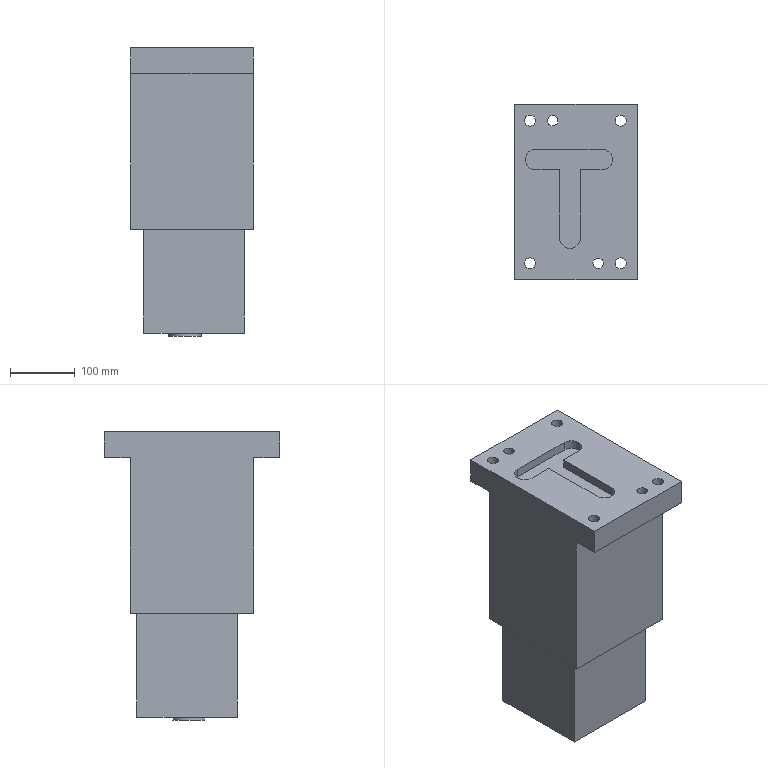Part | NX | features solid 2 | 1 solid | 42 faces | box 188.25 x 270 x 445 mm | volume 14281883 mm3 | plane 26 | cylinder 15 | cone 1 | commonest cylinder face diameters 17 x4 25 x4 32 x3 16 x2 20 x1 50 x1
STEP:
#1=CARTESIAN_POINT('',(-1140.,-620.,130.));
#2=VERTEX_POINT('',#1);
#3=CARTESIAN_POINT('',(-1140.,-350.,130.));
#4=VERTEX_POINT('',#3);
#5=CARTESIAN_POINT('',(-1140.,-555.,130.));
#6=DIRECTION('',(0.,-1.,0.));
#7=VECTOR('',#6,1000.);
#8=LINE('',#5,#7);
#9=EDGE_CURVE('',#2,#4,#8,.F.);
#10=ORIENTED_EDGE('',*,*,#9,.F.);
#11=CARTESIAN_POINT('',(-951.75,-620.,130.));
#12=VERTEX_POINT('',#11);
#13=CARTESIAN_POINT('',(-1136.75,-620.,130.));
#14=DIRECTION('',(1.,0.,0.));
#15=VECTOR('',#14,1000.);
#16=LINE('',#13,#15);
#17=EDGE_CURVE('',#2,#12,#16,.T.);
#18=ORIENTED_EDGE('',*,*,#17,.T.);
#19=CARTESIAN_POINT('',(-951.75,-350.,130.));
#20=VERTEX_POINT('',#19);
#21=CARTESIAN_POINT('',(-951.75,-564.335,130.));
#22=DIRECTION('',(0.,1.,0.));
#23=VECTOR('',#22,1000.);
#24=LINE('',#21,#23);
#25=EDGE_CURVE('',#12,#20,#24,.T.);
#26=ORIENTED_EDGE('',*,*,#25,.T.);
#27=CARTESIAN_POINT('',(-1136.75,-350.,130.));
#28=DIRECTION('',(-1.,0.,0.));
#29=VECTOR('',#28,1000.);
#30=LINE('',#27,#29);
#31=EDGE_CURVE('',#20,#4,#30,.T.);
#32=ORIENTED_EDGE('',*,*,#31,.T.);
#33=EDGE_LOOP('',(#10,#18,#26,#32));
#34=FACE_BOUND('',#33,.T.);
#35=CARTESIAN_POINT('',(-1019.75,-595.,130.));
#36=VERTEX_POINT('',#35);
#37=CARTESIAN_POINT('',(-1011.75,-595.,130.));
#38=DIRECTION('',(0.,0.,-1.));
#39=DIRECTION('',(-1.,0.,0.));
#40=AXIS2_PLACEMENT_3D('',#37,#38,#39);
#41=CIRCLE('',#40,8.);
#42=EDGE_CURVE('',#36,#36,#41,.T.);
#43=ORIENTED_EDGE('',*,*,#42,.T.);
#44=EDGE_LOOP('',(#43));
#45=FACE_BOUND('',#44,.T.);
#46=CARTESIAN_POINT('',(-985.25,-595.,130.));
#47=VERTEX_POINT('',#46);
#48=CARTESIAN_POINT('',(-976.75,-595.,130.));
#49=DIRECTION('',(0.,0.,-1.));
#50=DIRECTION('',(-1.,0.,0.));
#51=AXIS2_PLACEMENT_3D('',#48,#49,#50);
#52=CIRCLE('',#51,8.5);
#53=EDGE_CURVE('',#47,#47,#52,.T.);
#54=ORIENTED_EDGE('',*,*,#53,.T.);
#55=EDGE_LOOP('',(#54));
#56=FACE_BOUND('',#55,.T.);
#57=CARTESIAN_POINT('',(-985.25,-375.,130.));
#58=VERTEX_POINT('',#57);
#59=CARTESIAN_POINT('',(-976.75,-375.,130.));
#60=DIRECTION('',(0.,0.,-1.));
#61=DIRECTION('',(-1.,0.,0.));
#62=AXIS2_PLACEMENT_3D('',#59,#60,#61);
#63=CIRCLE('',#62,8.5);
#64=EDGE_CURVE('',#58,#58,#63,.T.);
#65=ORIENTED_EDGE('',*,*,#64,.T.);
#66=EDGE_LOOP('',(#65));
#67=FACE_BOUND('',#66,.T.);
#68=CARTESIAN_POINT('',(-1071.,-556.,130.));
#69=VERTEX_POINT('',#68);
#70=CARTESIAN_POINT('',(-1071.,-451.,130.));
#71=VERTEX_POINT('',#70);
#72=CARTESIAN_POINT('',(-1071.,-564.335,130.));
#73=DIRECTION('',(0.,-1.,0.));
#74=VECTOR('',#73,1000.);
#75=LINE('',#72,#74);
#76=EDGE_CURVE('',#69,#71,#75,.F.);
#77=ORIENTED_EDGE('',*,*,#76,.T.);
#78=CARTESIAN_POINT('',(-1107.75,-451.,130.));
#79=VERTEX_POINT('',#78);
#80=CARTESIAN_POINT('',(-1061.75,-451.,130.));
#81=DIRECTION('',(1.,0.,0.));
#82=VECTOR('',#81,1000.);
#83=LINE('',#80,#82);
#84=EDGE_CURVE('',#79,#71,#83,.T.);
#85=ORIENTED_EDGE('',*,*,#84,.F.);
#86=CARTESIAN_POINT('',(-1107.75,-419.,130.));
#87=VERTEX_POINT('',#86);
#88=CARTESIAN_POINT('',(-1107.75,-435.,130.));
#89=DIRECTION('',(0.,0.,-1.));
#90=DIRECTION('',(-1.,0.,0.));
#91=AXIS2_PLACEMENT_3D('',#88,#89,#90);
#92=CIRCLE('',#91,16.);
#93=EDGE_CURVE('',#79,#87,#92,.T.);
#94=ORIENTED_EDGE('',*,*,#93,.T.);
#95=CARTESIAN_POINT('',(-1005.75,-419.,130.));
#96=VERTEX_POINT('',#95);
#97=CARTESIAN_POINT('',(-1126.75,-419.,130.));
#98=DIRECTION('',(1.,0.,0.));
#99=VECTOR('',#98,1000.);
#100=LINE('',#97,#99);
#101=EDGE_CURVE('',#87,#96,#100,.T.);
#102=ORIENTED_EDGE('',*,*,#101,.T.);
#103=CARTESIAN_POINT('',(-1005.75,-451.,130.));
#104=VERTEX_POINT('',#103);
#105=CARTESIAN_POINT('',(-1005.75,-435.,130.));
#106=DIRECTION('',(0.,0.,-1.));
#107=DIRECTION('',(-1.,0.,0.));
#108=AXIS2_PLACEMENT_3D('',#105,#106,#107);
#109=CIRCLE('',#108,16.);
#110=EDGE_CURVE('',#96,#104,#109,.T.);
#111=ORIENTED_EDGE('',*,*,#110,.T.);
#112=CARTESIAN_POINT('',(-1039.,-451.,130.));
#113=VERTEX_POINT('',#112);
#114=CARTESIAN_POINT('',(-1061.75,-451.,130.));
#115=DIRECTION('',(1.,0.,0.));
#116=VECTOR('',#115,1000.);
#117=LINE('',#114,#116);
#118=EDGE_CURVE('',#113,#104,#117,.T.);
#119=ORIENTED_EDGE('',*,*,#118,.F.);
#120=CARTESIAN_POINT('',(-1039.,-556.,130.));
#121=VERTEX_POINT('',#120);
#122=CARTESIAN_POINT('',(-1039.,-564.335,130.));
#123=DIRECTION('',(0.,-1.,0.));
#124=VECTOR('',#123,1000.);
#125=LINE('',#122,#124);
#126=EDGE_CURVE('',#113,#121,#125,.T.);
#127=ORIENTED_EDGE('',*,*,#126,.T.);
#128=CARTESIAN_POINT('',(-1055.,-556.,130.));
#129=DIRECTION('',(0.,0.,-1.));
#130=DIRECTION('',(-1.,0.,0.));
#131=AXIS2_PLACEMENT_3D('',#128,#129,#130);
#132=CIRCLE('',#131,16.);
#133=EDGE_CURVE('',#69,#121,#132,.F.);
#134=ORIENTED_EDGE('',*,*,#133,.F.);
#135=EDGE_LOOP('',(#77,#85,#94,#102,#111,#119,#127,#134));
#136=FACE_BOUND('',#135,.T.);
#137=CARTESIAN_POINT('',(-1125.25,-595.,130.));
#138=VERTEX_POINT('',#137);
#139=CARTESIAN_POINT('',(-1116.75,-595.,130.));
#140=DIRECTION('',(0.,0.,-1.));
#141=DIRECTION('',(-1.,0.,0.));
#142=AXIS2_PLACEMENT_3D('',#139,#140,#141);
#143=CIRCLE('',#142,8.5);
#144=EDGE_CURVE('',#138,#138,#143,.T.);
#145=ORIENTED_EDGE('',*,*,#144,.T.);
#146=EDGE_LOOP('',(#145));
#147=FACE_BOUND('',#146,.T.);
#148=CARTESIAN_POINT('',(-1125.25,-375.,130.));
#149=VERTEX_POINT('',#148);
#150=CARTESIAN_POINT('',(-1116.75,-375.,130.));
#151=DIRECTION('',(0.,0.,-1.));
#152=DIRECTION('',(-1.,0.,0.));
#153=AXIS2_PLACEMENT_3D('',#150,#151,#152);
#154=CIRCLE('',#153,8.5);
#155=EDGE_CURVE('',#149,#149,#154,.T.);
#156=ORIENTED_EDGE('',*,*,#155,.T.);
#157=EDGE_LOOP('',(#156));
#158=FACE_BOUND('',#157,.T.);
#159=CARTESIAN_POINT('',(-1073.75,-375.,130.));
#160=VERTEX_POINT('',#159);
#161=CARTESIAN_POINT('',(-1081.75,-375.,130.));
#162=DIRECTION('',(0.,0.,1.));
#163=DIRECTION('',(1.,0.,0.));
#164=AXIS2_PLACEMENT_3D('',#161,#162,#163);
#165=CIRCLE('',#164,8.);
#166=EDGE_CURVE('',#160,#160,#165,.F.);
#167=ORIENTED_EDGE('',*,*,#166,.T.);
#168=EDGE_LOOP('',(#167));
#169=FACE_BOUND('',#168,.T.);
#170=CARTESIAN_POINT('',(-1136.75,-564.335,130.));
#171=DIRECTION('',(0.,0.,1.));
#172=DIRECTION('',(0.,-1.,0.));
#173=AXIS2_PLACEMENT_3D('',#170,#171,#172);
#174=PLANE('',#173);
#175=ADVANCED_FACE('',(#34,#45,#56,#67,#136,#147,#158,#169),#174,.T.);
#176=CARTESIAN_POINT('',(-951.75,-350.,90.));
#177=VERTEX_POINT('',#176);
#178=CARTESIAN_POINT('',(-951.75,-390.,90.));
#179=VERTEX_POINT('',#178);
#180=CARTESIAN_POINT('',(-951.75,-484.335,90.));
#181=DIRECTION('',(0.,-1.,0.));
#182=VECTOR('',#181,1000.);
#183=LINE('',#180,#182);
#184=EDGE_CURVE('',#177,#179,#183,.T.);
#185=ORIENTED_EDGE('',*,*,#184,.T.);
#186=CARTESIAN_POINT('',(-1140.,-390.,90.));
#187=VERTEX_POINT('',#186);
#188=CARTESIAN_POINT('',(-974.25,-390.,90.));
#189=DIRECTION('',(-1.,0.,0.));
#190=VECTOR('',#189,1000.);
#191=LINE('',#188,#190);
#192=EDGE_CURVE('',#179,#187,#191,.T.);
#193=ORIENTED_EDGE('',*,*,#192,.T.);
#194=CARTESIAN_POINT('',(-1140.,-350.,90.));
#195=VERTEX_POINT('',#194);
#196=CARTESIAN_POINT('',(-1140.,-555.,90.));
#197=DIRECTION('',(0.,1.,0.));
#198=VECTOR('',#197,1000.);
#199=LINE('',#196,#198);
#200=EDGE_CURVE('',#195,#187,#199,.F.);
#201=ORIENTED_EDGE('',*,*,#200,.F.);
#202=CARTESIAN_POINT('',(-974.25,-350.,90.));
#203=DIRECTION('',(-1.,0.,0.));
#204=VECTOR('',#203,1000.);
#205=LINE('',#202,#204);
#206=EDGE_CURVE('',#177,#195,#205,.T.);
#207=ORIENTED_EDGE('',*,*,#206,.F.);
#208=EDGE_LOOP('',(#185,#193,#201,#207));
#209=FACE_BOUND('',#208,.T.);
#210=CARTESIAN_POINT('',(-989.25,-375.,90.));
#211=VERTEX_POINT('',#210);
#212=CARTESIAN_POINT('',(-976.75,-375.,90.));
#213=DIRECTION('',(0.,0.,-1.));
#214=DIRECTION('',(-1.,0.,0.));
#215=AXIS2_PLACEMENT_3D('',#212,#213,#214);
#216=CIRCLE('',#215,12.5);
#217=EDGE_CURVE('',#211,#211,#216,.T.);
#218=ORIENTED_EDGE('',*,*,#217,.F.);
#219=EDGE_LOOP('',(#218));
#220=FACE_BOUND('',#219,.T.);
#221=CARTESIAN_POINT('',(-1104.25,-375.,90.));
#222=VERTEX_POINT('',#221);
#223=CARTESIAN_POINT('',(-1116.75,-375.,90.));
#224=DIRECTION('',(0.,0.,1.));
#225=DIRECTION('',(1.,0.,0.));
#226=AXIS2_PLACEMENT_3D('',#223,#224,#225);
#227=CIRCLE('',#226,12.5);
#228=EDGE_CURVE('',#222,#222,#227,.T.);
#229=ORIENTED_EDGE('',*,*,#228,.T.);
#230=EDGE_LOOP('',(#229));
#231=FACE_BOUND('',#230,.T.);
#232=CARTESIAN_POINT('',(-1089.75,-375.,90.));
#233=VERTEX_POINT('',#232);
#234=CARTESIAN_POINT('',(-1081.75,-375.,90.));
#235=DIRECTION('',(0.,0.,-1.));
#236=DIRECTION('',(-1.,0.,0.));
#237=AXIS2_PLACEMENT_3D('',#234,#235,#236);
#238=CIRCLE('',#237,8.);
#239=EDGE_CURVE('',#233,#233,#238,.F.);
#240=ORIENTED_EDGE('',*,*,#239,.T.);
#241=EDGE_LOOP('',(#240));
#242=FACE_BOUND('',#241,.T.);
#243=CARTESIAN_POINT('',(-974.25,-484.335,90.));
#244=DIRECTION('',(0.,0.,-1.));
#245=DIRECTION('',(-1.,0.,0.));
#246=AXIS2_PLACEMENT_3D('',#243,#244,#245);
#247=PLANE('',#246);
#248=ADVANCED_FACE('',(#209,#220,#231,#242),#247,.T.);
#249=CARTESIAN_POINT('',(-1120.,-400.,-150.));
#250=VERTEX_POINT('',#249);
#251=CARTESIAN_POINT('',(-965.,-400.,-150.));
#252=VERTEX_POINT('',#251);
#253=CARTESIAN_POINT('',(-861.25,-400.,-150.));
#254=DIRECTION('',(-1.,0.,0.));
#255=VECTOR('',#254,1000.);
#256=LINE('',#253,#255);
#257=EDGE_CURVE('',#250,#252,#256,.F.);
#258=ORIENTED_EDGE('',*,*,#257,.T.);
#259=CARTESIAN_POINT('',(-965.,-400.,-310.));
#260=VERTEX_POINT('',#259);
#261=CARTESIAN_POINT('',(-965.,-400.,-100.));
#262=DIRECTION('',(0.,0.,-1.));
#263=VECTOR('',#262,1000.);
#264=LINE('',#261,#263);
#265=EDGE_CURVE('',#252,#260,#264,.T.);
#266=ORIENTED_EDGE('',*,*,#265,.T.);
#267=CARTESIAN_POINT('',(-1120.,-400.,-310.));
#268=VERTEX_POINT('',#267);
#269=CARTESIAN_POINT('',(-861.25,-400.,-310.));
#270=DIRECTION('',(1.,0.,0.));
#271=VECTOR('',#270,1000.);
#272=LINE('',#269,#271);
#273=EDGE_CURVE('',#260,#268,#272,.F.);
#274=ORIENTED_EDGE('',*,*,#273,.T.);
#275=CARTESIAN_POINT('',(-1120.,-400.,-95.));
#276=DIRECTION('',(0.,0.,-1.));
#277=VECTOR('',#276,1000.);
#278=LINE('',#275,#277);
#279=EDGE_CURVE('',#250,#268,#278,.T.);
#280=ORIENTED_EDGE('',*,*,#279,.F.);
#281=EDGE_LOOP('',(#258,#266,#274,#280));
#282=FACE_BOUND('',#281,.T.);
#283=CARTESIAN_POINT('',(-861.25,-400.,-95.));
#284=DIRECTION('',(0.,1.,0.));
#285=DIRECTION('',(0.,0.,-1.));
#286=AXIS2_PLACEMENT_3D('',#283,#284,#285);
#287=PLANE('',#286);
#288=ADVANCED_FACE('',(#282),#287,.T.);
#289=CARTESIAN_POINT('',(-1081.75,-480.,-310.));
#290=VERTEX_POINT('',#289);
#291=CARTESIAN_POINT('',(-1056.75,-480.,-310.));
#292=DIRECTION('',(0.,0.,1.));
#293=DIRECTION('',(-1.,0.,0.));
#294=AXIS2_PLACEMENT_3D('',#291,#292,#293);
#295=CIRCLE('',#294,25.);
#296=EDGE_CURVE('',#290,#290,#295,.F.);
#297=ORIENTED_EDGE('',*,*,#296,.F.);
#298=EDGE_LOOP('',(#297));
#299=FACE_BOUND('',#298,.T.);
#300=ORIENTED_EDGE('',*,*,#273,.F.);
#301=CARTESIAN_POINT('',(-965.,-555.,-310.));
#302=VERTEX_POINT('',#301);
#303=CARTESIAN_POINT('',(-965.,-554.793,-310.));
#304=DIRECTION('',(0.,1.,0.));
#305=VECTOR('',#304,1000.);
#306=LINE('',#303,#305);
#307=EDGE_CURVE('',#260,#302,#306,.F.);
#308=ORIENTED_EDGE('',*,*,#307,.T.);
#309=CARTESIAN_POINT('',(-1120.,-555.,-310.));
#310=VERTEX_POINT('',#309);
#311=CARTESIAN_POINT('',(-1089.25,-555.,-310.));
#312=DIRECTION('',(-1.,0.,0.));
#313=VECTOR('',#312,1000.);
#314=LINE('',#311,#313);
#315=EDGE_CURVE('',#310,#302,#314,.F.);
#316=ORIENTED_EDGE('',*,*,#315,.F.);
#317=CARTESIAN_POINT('',(-1120.,-510.347,-310.));
#318=DIRECTION('',(0.,1.,0.));
#319=VECTOR('',#318,1000.);
#320=LINE('',#317,#319);
#321=EDGE_CURVE('',#268,#310,#320,.F.);
#322=ORIENTED_EDGE('',*,*,#321,.F.);
#323=EDGE_LOOP('',(#300,#308,#316,#322));
#324=FACE_BOUND('',#323,.T.);
#325=CARTESIAN_POINT('',(249.,-554.793,-310.));
#326=DIRECTION('',(0.,0.,-1.));
#327=DIRECTION('',(-1.,0.,0.));
#328=AXIS2_PLACEMENT_3D('',#325,#326,#327);
#329=PLANE('',#328);
#330=ADVANCED_FACE('',(#299,#324),#329,.T.);
#331=CARTESIAN_POINT('',(-1120.,-555.,-150.));
#332=VERTEX_POINT('',#331);
#333=CARTESIAN_POINT('',(-1120.,-489.988,-150.));
#334=DIRECTION('',(0.,1.,0.));
#335=VECTOR('',#334,1000.);
#336=LINE('',#333,#335);
#337=EDGE_CURVE('',#250,#332,#336,.F.);
#338=ORIENTED_EDGE('',*,*,#337,.T.);
#339=CARTESIAN_POINT('',(-965.,-555.,-150.));
#340=VERTEX_POINT('',#339);
#341=CARTESIAN_POINT('',(-1243.183,-555.,-150.));
#342=DIRECTION('',(-1.,0.,0.));
#343=VECTOR('',#342,1000.);
#344=LINE('',#341,#343);
#345=EDGE_CURVE('',#332,#340,#344,.F.);
#346=ORIENTED_EDGE('',*,*,#345,.T.);
#347=CARTESIAN_POINT('',(-965.,-489.988,-150.));
#348=DIRECTION('',(0.,-1.,0.));
#349=VECTOR('',#348,1000.);
#350=LINE('',#347,#349);
#351=EDGE_CURVE('',#340,#252,#350,.F.);
#352=ORIENTED_EDGE('',*,*,#351,.T.);
#353=ORIENTED_EDGE('',*,*,#257,.F.);
#354=EDGE_LOOP('',(#338,#346,#352,#353));
#355=FACE_BOUND('',#354,.T.);
#356=CARTESIAN_POINT('',(-1140.,-580.,-150.));
#357=VERTEX_POINT('',#356);
#358=CARTESIAN_POINT('',(-951.75,-580.,-150.));
#359=VERTEX_POINT('',#358);
#360=CARTESIAN_POINT('',(-1136.75,-580.,-150.));
#361=DIRECTION('',(1.,0.,0.));
#362=VECTOR('',#361,1000.);
#363=LINE('',#360,#362);
#364=EDGE_CURVE('',#357,#359,#363,.T.);
#365=ORIENTED_EDGE('',*,*,#364,.F.);
#366=CARTESIAN_POINT('',(-1140.,-390.,-150.));
#367=VERTEX_POINT('',#366);
#368=CARTESIAN_POINT('',(-1140.,-555.,-150.));
#369=DIRECTION('',(0.,-1.,0.));
#370=VECTOR('',#369,1000.);
#371=LINE('',#368,#370);
#372=EDGE_CURVE('',#367,#357,#371,.T.);
#373=ORIENTED_EDGE('',*,*,#372,.F.);
#374=CARTESIAN_POINT('',(-951.75,-390.,-150.));
#375=VERTEX_POINT('',#374);
#376=CARTESIAN_POINT('',(-1089.25,-390.,-150.));
#377=DIRECTION('',(-1.,0.,0.));
#378=VECTOR('',#377,1000.);
#379=LINE('',#376,#378);
#380=EDGE_CURVE('',#367,#375,#379,.F.);
#381=ORIENTED_EDGE('',*,*,#380,.T.);
#382=CARTESIAN_POINT('',(-951.75,-484.335,-150.));
#383=DIRECTION('',(0.,-1.,0.));
#384=VECTOR('',#383,1000.);
#385=LINE('',#382,#384);
#386=EDGE_CURVE('',#359,#375,#385,.F.);
#387=ORIENTED_EDGE('',*,*,#386,.F.);
#388=EDGE_LOOP('',(#365,#373,#381,#387));
#389=FACE_BOUND('',#388,.T.);
#390=CARTESIAN_POINT('',(-1243.183,-489.988,-150.));
#391=DIRECTION('',(0.,0.,1.));
#392=DIRECTION('',(-0.342,0.9397,0.));
#393=AXIS2_PLACEMENT_3D('',#390,#391,#392);
#394=PLANE('',#393);
#395=ADVANCED_FACE('',(#355,#389),#394,.F.);
#396=ORIENTED_EDGE('',*,*,#372,.T.);
#397=CARTESIAN_POINT('',(-1140.,-580.,90.));
#398=VERTEX_POINT('',#397);
#399=CARTESIAN_POINT('',(-1140.,-580.,-150.));
#400=DIRECTION('',(0.,0.,1.));
#401=VECTOR('',#400,1000.);
#402=LINE('',#399,#401);
#403=EDGE_CURVE('',#357,#398,#402,.T.);
#404=ORIENTED_EDGE('',*,*,#403,.T.);
#405=CARTESIAN_POINT('',(-1140.,-620.,90.));
#406=VERTEX_POINT('',#405);
#407=CARTESIAN_POINT('',(-1140.,-555.,90.));
#408=DIRECTION('',(0.,1.,0.));
#409=VECTOR('',#408,1000.);
#410=LINE('',#407,#409);
#411=EDGE_CURVE('',#406,#398,#410,.T.);
#412=ORIENTED_EDGE('',*,*,#411,.F.);
#413=CARTESIAN_POINT('',(-1140.,-620.,-300.));
#414=DIRECTION('',(0.,0.,1.));
#415=VECTOR('',#414,1000.);
#416=LINE('',#413,#415);
#417=EDGE_CURVE('',#2,#406,#416,.F.);
#418=ORIENTED_EDGE('',*,*,#417,.F.);
#419=ORIENTED_EDGE('',*,*,#9,.T.);
#420=CARTESIAN_POINT('',(-1140.,-350.,-300.));
#421=DIRECTION('',(0.,0.,-1.));
#422=VECTOR('',#421,1000.);
#423=LINE('',#420,#422);
#424=EDGE_CURVE('',#195,#4,#423,.F.);
#425=ORIENTED_EDGE('',*,*,#424,.F.);
#426=ORIENTED_EDGE('',*,*,#200,.T.);
#427=CARTESIAN_POINT('',(-1140.,-390.,-300.));
#428=DIRECTION('',(0.,0.,1.));
#429=VECTOR('',#428,1000.);
#430=LINE('',#427,#429);
#431=EDGE_CURVE('',#187,#367,#430,.F.);
#432=ORIENTED_EDGE('',*,*,#431,.T.);
#433=EDGE_LOOP('',(#396,#404,#412,#418,#419,#425,#426,#432));
#434=FACE_BOUND('',#433,.T.);
#435=CARTESIAN_POINT('',(-1140.,-555.,-300.));
#436=DIRECTION('',(-1.,0.,0.));
#437=DIRECTION('',(0.,0.,1.));
#438=AXIS2_PLACEMENT_3D('',#435,#436,#437);
#439=PLANE('',#438);
#440=ADVANCED_FACE('',(#434),#439,.T.);
#441=CARTESIAN_POINT('',(-1120.,-555.,-150.));
#442=DIRECTION('',(0.,0.,-1.));
#443=VECTOR('',#442,1000.);
#444=LINE('',#441,#443);
#445=EDGE_CURVE('',#332,#310,#444,.T.);
#446=ORIENTED_EDGE('',*,*,#445,.T.);
#447=ORIENTED_EDGE('',*,*,#315,.T.);
#448=CARTESIAN_POINT('',(-965.,-555.,-155.));
#449=DIRECTION('',(0.,0.,-1.));
#450=VECTOR('',#449,1000.);
#451=LINE('',#448,#450);
#452=EDGE_CURVE('',#340,#302,#451,.T.);
#453=ORIENTED_EDGE('',*,*,#452,.F.);
#454=ORIENTED_EDGE('',*,*,#345,.F.);
#455=EDGE_LOOP('',(#446,#447,#453,#454));
#456=FACE_BOUND('',#455,.T.);
#457=CARTESIAN_POINT('',(-1089.25,-555.,-155.));
#458=DIRECTION('',(0.,-1.,0.));
#459=DIRECTION('',(1.,0.,0.));
#460=AXIS2_PLACEMENT_3D('',#457,#458,#459);
#461=PLANE('',#460);
#462=ADVANCED_FACE('',(#456),#461,.T.);
#463=ORIENTED_EDGE('',*,*,#452,.T.);
#464=ORIENTED_EDGE('',*,*,#307,.F.);
#465=ORIENTED_EDGE('',*,*,#265,.F.);
#466=ORIENTED_EDGE('',*,*,#351,.F.);
#467=EDGE_LOOP('',(#463,#464,#465,#466));
#468=FACE_BOUND('',#467,.T.);
#469=CARTESIAN_POINT('',(-965.,-517.5,-100.));
#470=DIRECTION('',(1.,0.,0.));
#471=DIRECTION('',(0.,0.,-1.));
#472=AXIS2_PLACEMENT_3D('',#469,#470,#471);
#473=PLANE('',#472);
#474=ADVANCED_FACE('',(#468),#473,.T.);
#475=CARTESIAN_POINT('',(-951.75,-580.,90.));
#476=VERTEX_POINT('',#475);
#477=CARTESIAN_POINT('',(-951.75,-580.,-150.));
#478=DIRECTION('',(0.,0.,1.));
#479=VECTOR('',#478,1000.);
#480=LINE('',#477,#479);
#481=EDGE_CURVE('',#359,#476,#480,.T.);
#482=ORIENTED_EDGE('',*,*,#481,.T.);
#483=CARTESIAN_POINT('',(-974.25,-580.,90.));
#484=DIRECTION('',(1.,0.,0.));
#485=VECTOR('',#484,1000.);
#486=LINE('',#483,#485);
#487=EDGE_CURVE('',#398,#476,#486,.T.);
#488=ORIENTED_EDGE('',*,*,#487,.F.);
#489=ORIENTED_EDGE('',*,*,#403,.F.);
#490=ORIENTED_EDGE('',*,*,#364,.T.);
#491=EDGE_LOOP('',(#482,#488,#489,#490));
#492=FACE_BOUND('',#491,.T.);
#493=CARTESIAN_POINT('',(-1136.75,-580.,-150.));
#494=DIRECTION('',(0.,-1.,0.));
#495=DIRECTION('',(1.,0.,0.));
#496=AXIS2_PLACEMENT_3D('',#493,#494,#495);
#497=PLANE('',#496);
#498=ADVANCED_FACE('',(#492),#497,.T.);
#499=CARTESIAN_POINT('',(-1039.,-556.,116.));
#500=VERTEX_POINT('',#499);
#501=CARTESIAN_POINT('',(-1039.,-451.,116.));
#502=VERTEX_POINT('',#501);
#503=CARTESIAN_POINT('',(-1039.,-534.335,116.));
#504=DIRECTION('',(0.,1.,0.));
#505=VECTOR('',#504,1000.);
#506=LINE('',#503,#505);
#507=EDGE_CURVE('',#500,#502,#506,.T.);
#508=ORIENTED_EDGE('',*,*,#507,.T.);
#509=CARTESIAN_POINT('',(-1005.75,-451.,116.));
#510=VERTEX_POINT('',#509);
#511=CARTESIAN_POINT('',(-1061.75,-451.,116.));
#512=DIRECTION('',(1.,0.,0.));
#513=VECTOR('',#512,1000.);
#514=LINE('',#511,#513);
#515=EDGE_CURVE('',#502,#510,#514,.T.);
#516=ORIENTED_EDGE('',*,*,#515,.T.);
#517=CARTESIAN_POINT('',(-1005.75,-419.,116.));
#518=VERTEX_POINT('',#517);
#519=CARTESIAN_POINT('',(-1005.75,-435.,116.));
#520=DIRECTION('',(0.,0.,1.));
#521=DIRECTION('',(-1.,0.,0.));
#522=AXIS2_PLACEMENT_3D('',#519,#520,#521);
#523=CIRCLE('',#522,16.);
#524=EDGE_CURVE('',#518,#510,#523,.F.);
#525=ORIENTED_EDGE('',*,*,#524,.F.);
#526=CARTESIAN_POINT('',(-1107.75,-419.,116.));
#527=VERTEX_POINT('',#526);
#528=CARTESIAN_POINT('',(-1061.75,-419.,116.));
#529=DIRECTION('',(1.,0.,0.));
#530=VECTOR('',#529,1000.);
#531=LINE('',#528,#530);
#532=EDGE_CURVE('',#527,#518,#531,.T.);
#533=ORIENTED_EDGE('',*,*,#532,.F.);
#534=CARTESIAN_POINT('',(-1107.75,-451.,116.));
#535=VERTEX_POINT('',#534);
#536=CARTESIAN_POINT('',(-1107.75,-435.,116.));
#537=DIRECTION('',(0.,0.,1.));
#538=DIRECTION('',(-1.,0.,0.));
#539=AXIS2_PLACEMENT_3D('',#536,#537,#538);
#540=CIRCLE('',#539,16.);
#541=EDGE_CURVE('',#535,#527,#540,.F.);
#542=ORIENTED_EDGE('',*,*,#541,.F.);
#543=CARTESIAN_POINT('',(-1071.,-451.,116.));
#544=VERTEX_POINT('',#543);
#545=CARTESIAN_POINT('',(-1061.75,-451.,116.));
#546=DIRECTION('',(1.,0.,0.));
#547=VECTOR('',#546,1000.);
#548=LINE('',#545,#547);
#549=EDGE_CURVE('',#535,#544,#548,.T.);
#550=ORIENTED_EDGE('',*,*,#549,.T.);
#551=CARTESIAN_POINT('',(-1071.,-556.,116.));
#552=VERTEX_POINT('',#551);
#553=CARTESIAN_POINT('',(-1071.,-744.335,116.));
#554=DIRECTION('',(0.,-1.,0.));
#555=VECTOR('',#554,1000.);
#556=LINE('',#553,#555);
#557=EDGE_CURVE('',#552,#544,#556,.F.);
#558=ORIENTED_EDGE('',*,*,#557,.F.);
#559=CARTESIAN_POINT('',(-1055.,-556.,116.));
#560=DIRECTION('',(0.,0.,1.));
#561=DIRECTION('',(-1.,0.,0.));
#562=AXIS2_PLACEMENT_3D('',#559,#560,#561);
#563=CIRCLE('',#562,16.);
#564=EDGE_CURVE('',#500,#552,#563,.F.);
#565=ORIENTED_EDGE('',*,*,#564,.F.);
#566=EDGE_LOOP('',(#508,#516,#525,#533,#542,#550,#558,#565));
#567=FACE_BOUND('',#566,.T.);
#568=CARTESIAN_POINT('',(-1071.75,-534.335,116.));
#569=DIRECTION('',(0.,0.,-1.));
#570=DIRECTION('',(-1.,0.,0.));
#571=AXIS2_PLACEMENT_3D('',#568,#569,#570);
#572=PLANE('',#571);
#573=ADVANCED_FACE('',(#567),#572,.F.);
#574=ORIENTED_EDGE('',*,*,#557,.T.);
#575=CARTESIAN_POINT('',(-1071.,-451.,115.));
#576=DIRECTION('',(0.,0.,-1.));
#577=VECTOR('',#576,1000.);
#578=LINE('',#575,#577);
#579=EDGE_CURVE('',#544,#71,#578,.F.);
#580=ORIENTED_EDGE('',*,*,#579,.T.);
#581=ORIENTED_EDGE('',*,*,#76,.F.);
#582=CARTESIAN_POINT('',(-1071.,-556.,100.));
#583=DIRECTION('',(0.,0.,-1.));
#584=VECTOR('',#583,1000.);
#585=LINE('',#582,#584);
#586=EDGE_CURVE('',#552,#69,#585,.F.);
#587=ORIENTED_EDGE('',*,*,#586,.F.);
#588=EDGE_LOOP('',(#574,#580,#581,#587));
#589=FACE_BOUND('',#588,.T.);
#590=CARTESIAN_POINT('',(-1071.,-744.335,100.));
#591=DIRECTION('',(1.,0.,0.));
#592=DIRECTION('',(0.,1.,0.));
#593=AXIS2_PLACEMENT_3D('',#590,#591,#592);
#594=PLANE('',#593);
#595=ADVANCED_FACE('',(#589),#594,.T.);
#596=ORIENTED_EDGE('',*,*,#126,.F.);
#597=CARTESIAN_POINT('',(-1039.,-451.,100.));
#598=DIRECTION('',(0.,0.,1.));
#599=VECTOR('',#598,1000.);
#600=LINE('',#597,#599);
#601=EDGE_CURVE('',#502,#113,#600,.T.);
#602=ORIENTED_EDGE('',*,*,#601,.F.);
#603=ORIENTED_EDGE('',*,*,#507,.F.);
#604=CARTESIAN_POINT('',(-1039.,-556.,100.));
#605=DIRECTION('',(0.,0.,-1.));
#606=VECTOR('',#605,1000.);
#607=LINE('',#604,#606);
#608=EDGE_CURVE('',#121,#500,#607,.T.);
#609=ORIENTED_EDGE('',*,*,#608,.F.);
#610=EDGE_LOOP('',(#596,#602,#603,#609));
#611=FACE_BOUND('',#610,.T.);
#612=CARTESIAN_POINT('',(-1039.,-744.335,100.));
#613=DIRECTION('',(1.,0.,0.));
#614=DIRECTION('',(0.,1.,0.));
#615=AXIS2_PLACEMENT_3D('',#612,#613,#614);
#616=PLANE('',#615);
#617=ADVANCED_FACE('',(#611),#616,.F.);
#618=ORIENTED_EDGE('',*,*,#380,.F.);
#619=ORIENTED_EDGE('',*,*,#431,.F.);
#620=ORIENTED_EDGE('',*,*,#192,.F.);
#621=CARTESIAN_POINT('',(-951.75,-390.,-153.));
#622=DIRECTION('',(0.,0.,-1.));
#623=VECTOR('',#622,1000.);
#624=LINE('',#621,#623);
#625=EDGE_CURVE('',#375,#179,#624,.F.);
#626=ORIENTED_EDGE('',*,*,#625,.F.);
#627=EDGE_LOOP('',(#618,#619,#620,#626));
#628=FACE_BOUND('',#627,.T.);
#629=CARTESIAN_POINT('',(-1134.75,-390.,-153.));
#630=DIRECTION('',(0.,1.,0.));
#631=DIRECTION('',(1.,0.,0.));
#632=AXIS2_PLACEMENT_3D('',#629,#630,#631);
#633=PLANE('',#632);
#634=ADVANCED_FACE('',(#628),#633,.T.);
#635=ORIENTED_EDGE('',*,*,#549,.F.);
#636=CARTESIAN_POINT('',(-1107.75,-451.,115.));
#637=DIRECTION('',(0.,0.,1.));
#638=VECTOR('',#637,1000.);
#639=LINE('',#636,#638);
#640=EDGE_CURVE('',#535,#79,#639,.T.);
#641=ORIENTED_EDGE('',*,*,#640,.T.);
#642=ORIENTED_EDGE('',*,*,#84,.T.);
#643=ORIENTED_EDGE('',*,*,#579,.F.);
#644=EDGE_LOOP('',(#635,#641,#642,#643));
#645=FACE_BOUND('',#644,.T.);
#646=CARTESIAN_POINT('',(-1061.75,-451.,115.));
#647=DIRECTION('',(0.,-1.,0.));
#648=DIRECTION('',(0.,0.,1.));
#649=AXIS2_PLACEMENT_3D('',#646,#647,#648);
#650=PLANE('',#649);
#651=ADVANCED_FACE('',(#645),#650,.F.);
#652=CARTESIAN_POINT('',(-951.75,-620.,90.));
#653=VERTEX_POINT('',#652);
#654=CARTESIAN_POINT('',(-951.75,-620.,-75.));
#655=DIRECTION('',(0.,0.,1.));
#656=VECTOR('',#655,1000.);
#657=LINE('',#654,#656);
#658=EDGE_CURVE('',#653,#12,#657,.T.);
#659=ORIENTED_EDGE('',*,*,#658,.T.);
#660=ORIENTED_EDGE('',*,*,#17,.F.);
#661=ORIENTED_EDGE('',*,*,#417,.T.);
#662=CARTESIAN_POINT('',(-974.25,-620.,90.));
#663=DIRECTION('',(-1.,0.,0.));
#664=VECTOR('',#663,1000.);
#665=LINE('',#662,#664);
#666=EDGE_CURVE('',#406,#653,#665,.F.);
#667=ORIENTED_EDGE('',*,*,#666,.T.);
#668=EDGE_LOOP('',(#659,#660,#661,#667));
#669=FACE_BOUND('',#668,.T.);
#670=CARTESIAN_POINT('',(-1136.75,-620.,115.));
#671=DIRECTION('',(0.,1.,0.));
#672=DIRECTION('',(0.,0.,-1.));
#673=AXIS2_PLACEMENT_3D('',#670,#671,#672);
#674=PLANE('',#673);
#675=ADVANCED_FACE('',(#669),#674,.F.);
#676=CARTESIAN_POINT('',(-1104.25,-595.,90.));
#677=VERTEX_POINT('',#676);
#678=CARTESIAN_POINT('',(-1116.75,-595.,90.));
#679=DIRECTION('',(0.,0.,1.));
#680=DIRECTION('',(1.,0.,0.));
#681=AXIS2_PLACEMENT_3D('',#678,#679,#680);
#682=CIRCLE('',#681,12.5);
#683=EDGE_CURVE('',#677,#677,#682,.F.);
#684=ORIENTED_EDGE('',*,*,#683,.F.);
#685=EDGE_LOOP('',(#684));
#686=FACE_BOUND('',#685,.T.);
#687=CARTESIAN_POINT('',(-1019.75,-595.,90.));
#688=VERTEX_POINT('',#687);
#689=CARTESIAN_POINT('',(-1011.75,-595.,90.));
#690=DIRECTION('',(0.,0.,1.));
#691=DIRECTION('',(-1.,0.,0.));
#692=AXIS2_PLACEMENT_3D('',#689,#690,#691);
#693=CIRCLE('',#692,8.);
#694=EDGE_CURVE('',#688,#688,#693,.F.);
#695=ORIENTED_EDGE('',*,*,#694,.F.);
#696=EDGE_LOOP('',(#695));
#697=FACE_BOUND('',#696,.T.);
#698=CARTESIAN_POINT('',(-989.25,-595.,90.));
#699=VERTEX_POINT('',#698);
#700=CARTESIAN_POINT('',(-976.75,-595.,90.));
#701=DIRECTION('',(0.,0.,1.));
#702=DIRECTION('',(-1.,0.,0.));
#703=AXIS2_PLACEMENT_3D('',#700,#701,#702);
#704=CIRCLE('',#703,12.5);
#705=EDGE_CURVE('',#699,#699,#704,.F.);
#706=ORIENTED_EDGE('',*,*,#705,.F.);
#707=EDGE_LOOP('',(#706));
#708=FACE_BOUND('',#707,.T.);
#709=ORIENTED_EDGE('',*,*,#487,.T.);
#710=CARTESIAN_POINT('',(-951.75,-555.,90.));
#711=DIRECTION('',(0.,1.,0.));
#712=VECTOR('',#711,1000.);
#713=LINE('',#710,#712);
#714=EDGE_CURVE('',#476,#653,#713,.F.);
#715=ORIENTED_EDGE('',*,*,#714,.T.);
#716=ORIENTED_EDGE('',*,*,#666,.F.);
#717=ORIENTED_EDGE('',*,*,#411,.T.);
#718=EDGE_LOOP('',(#709,#715,#716,#717));
#719=FACE_BOUND('',#718,.T.);
#720=CARTESIAN_POINT('',(-974.25,-484.335,90.));
#721=DIRECTION('',(0.,0.,-1.));
#722=DIRECTION('',(-1.,0.,0.));
#723=AXIS2_PLACEMENT_3D('',#720,#721,#722);
#724=PLANE('',#723);
#725=ADVANCED_FACE('',(#686,#697,#708,#719),#724,.T.);
#726=ORIENTED_EDGE('',*,*,#118,.T.);
#727=CARTESIAN_POINT('',(-1005.75,-451.,115.));
#728=DIRECTION('',(0.,0.,1.));
#729=VECTOR('',#728,1000.);
#730=LINE('',#727,#729);
#731=EDGE_CURVE('',#510,#104,#730,.T.);
#732=ORIENTED_EDGE('',*,*,#731,.F.);
#733=ORIENTED_EDGE('',*,*,#515,.F.);
#734=ORIENTED_EDGE('',*,*,#601,.T.);
#735=EDGE_LOOP('',(#726,#732,#733,#734));
#736=FACE_BOUND('',#735,.T.);
#737=CARTESIAN_POINT('',(-1061.75,-451.,115.));
#738=DIRECTION('',(0.,-1.,0.));
#739=DIRECTION('',(0.,0.,1.));
#740=AXIS2_PLACEMENT_3D('',#737,#738,#739);
#741=PLANE('',#740);
#742=ADVANCED_FACE('',(#736),#741,.F.);
#743=ORIENTED_EDGE('',*,*,#93,.F.);
#744=ORIENTED_EDGE('',*,*,#640,.F.);
#745=ORIENTED_EDGE('',*,*,#541,.T.);
#746=CARTESIAN_POINT('',(-1107.75,-419.,115.));
#747=DIRECTION('',(0.,0.,-1.));
#748=VECTOR('',#747,1000.);
#749=LINE('',#746,#748);
#750=EDGE_CURVE('',#527,#87,#749,.F.);
#751=ORIENTED_EDGE('',*,*,#750,.T.);
#752=EDGE_LOOP('',(#743,#744,#745,#751));
#753=FACE_BOUND('',#752,.T.);
#754=CARTESIAN_POINT('',(-1107.75,-435.,115.));
#755=DIRECTION('',(0.,0.,1.));
#756=DIRECTION('',(1.,0.,0.));
#757=AXIS2_PLACEMENT_3D('',#754,#755,#756);
#758=CYLINDRICAL_SURFACE('',#757,16.);
#759=ADVANCED_FACE('',(#753),#758,.F.);
#760=ORIENTED_EDGE('',*,*,#101,.F.);
#761=ORIENTED_EDGE('',*,*,#750,.F.);
#762=ORIENTED_EDGE('',*,*,#532,.T.);
#763=CARTESIAN_POINT('',(-1005.75,-419.,115.));
#764=DIRECTION('',(0.,0.,1.));
#765=VECTOR('',#764,1000.);
#766=LINE('',#763,#765);
#767=EDGE_CURVE('',#518,#96,#766,.T.);
#768=ORIENTED_EDGE('',*,*,#767,.T.);
#769=EDGE_LOOP('',(#760,#761,#762,#768));
#770=FACE_BOUND('',#769,.T.);
#771=CARTESIAN_POINT('',(-1061.75,-419.,115.));
#772=DIRECTION('',(0.,1.,0.));
#773=DIRECTION('',(0.,0.,-1.));
#774=AXIS2_PLACEMENT_3D('',#771,#772,#773);
#775=PLANE('',#774);
#776=ADVANCED_FACE('',(#770),#775,.F.);
#777=ORIENTED_EDGE('',*,*,#110,.F.);
#778=ORIENTED_EDGE('',*,*,#767,.F.);
#779=ORIENTED_EDGE('',*,*,#524,.T.);
#780=ORIENTED_EDGE('',*,*,#731,.T.);
#781=EDGE_LOOP('',(#777,#778,#779,#780));
#782=FACE_BOUND('',#781,.T.);
#783=CARTESIAN_POINT('',(-1005.75,-435.,115.));
#784=DIRECTION('',(0.,0.,1.));
#785=DIRECTION('',(1.,0.,0.));
#786=AXIS2_PLACEMENT_3D('',#783,#784,#785);
#787=CYLINDRICAL_SURFACE('',#786,16.);
#788=ADVANCED_FACE('',(#782),#787,.F.);
#789=ORIENTED_EDGE('',*,*,#31,.F.);
#790=CARTESIAN_POINT('',(-951.75,-350.,90.));
#791=DIRECTION('',(0.,0.,1.));
#792=VECTOR('',#791,1000.);
#793=LINE('',#790,#792);
#794=EDGE_CURVE('',#177,#20,#793,.T.);
#795=ORIENTED_EDGE('',*,*,#794,.F.);
#796=ORIENTED_EDGE('',*,*,#206,.T.);
#797=ORIENTED_EDGE('',*,*,#424,.T.);
#798=EDGE_LOOP('',(#789,#795,#796,#797));
#799=FACE_BOUND('',#798,.T.);
#800=CARTESIAN_POINT('',(-974.25,-350.,90.));
#801=DIRECTION('',(0.,-1.,0.));
#802=DIRECTION('',(0.,0.,-1.));
#803=AXIS2_PLACEMENT_3D('',#800,#801,#802);
#804=PLANE('',#803);
#805=ADVANCED_FACE('',(#799),#804,.F.);
#806=ORIENTED_EDGE('',*,*,#586,.T.);
#807=ORIENTED_EDGE('',*,*,#133,.T.);
#808=ORIENTED_EDGE('',*,*,#608,.T.);
#809=ORIENTED_EDGE('',*,*,#564,.T.);
#810=EDGE_LOOP('',(#806,#807,#808,#809));
#811=FACE_BOUND('',#810,.T.);
#812=CARTESIAN_POINT('',(-1055.,-556.,100.));
#813=DIRECTION('',(0.,0.,-1.));
#814=DIRECTION('',(1.,0.,0.));
#815=AXIS2_PLACEMENT_3D('',#812,#813,#814);
#816=CYLINDRICAL_SURFACE('',#815,16.);
#817=ADVANCED_FACE('',(#811),#816,.F.);
#818=ORIENTED_EDGE('',*,*,#386,.T.);
#819=ORIENTED_EDGE('',*,*,#625,.T.);
#820=ORIENTED_EDGE('',*,*,#184,.F.);
#821=ORIENTED_EDGE('',*,*,#794,.T.);
#822=ORIENTED_EDGE('',*,*,#25,.F.);
#823=ORIENTED_EDGE('',*,*,#658,.F.);
#824=ORIENTED_EDGE('',*,*,#714,.F.);
#825=ORIENTED_EDGE('',*,*,#481,.F.);
#826=EDGE_LOOP('',(#818,#819,#820,#821,#822,#823,#824,#825));
#827=FACE_BOUND('',#826,.T.);
#828=CARTESIAN_POINT('',(-951.75,-555.,-85.));
#829=DIRECTION('',(-1.,0.,0.));
#830=DIRECTION('',(0.,0.,-1.));
#831=AXIS2_PLACEMENT_3D('',#828,#829,#830);
#832=PLANE('',#831);
#833=ADVANCED_FACE('',(#827),#832,.F.);
#834=ORIENTED_EDGE('',*,*,#64,.F.);
#835=EDGE_LOOP('',(#834));
#836=FACE_BOUND('',#835,.T.);
#837=CARTESIAN_POINT('',(-968.25,-375.,110.));
#838=VERTEX_POINT('',#837);
#839=CARTESIAN_POINT('',(-976.75,-375.,110.));
#840=DIRECTION('',(0.,0.,-1.));
#841=DIRECTION('',(1.,0.,0.));
#842=AXIS2_PLACEMENT_3D('',#839,#840,#841);
#843=CIRCLE('',#842,8.5);
#844=EDGE_CURVE('',#838,#838,#843,.T.);
#845=ORIENTED_EDGE('',*,*,#844,.T.);
#846=EDGE_LOOP('',(#845));
#847=FACE_BOUND('',#846,.T.);
#848=CARTESIAN_POINT('',(-976.75,-375.,140.));
#849=DIRECTION('',(0.,0.,1.));
#850=DIRECTION('',(-1.,0.,0.));
#851=AXIS2_PLACEMENT_3D('',#848,#849,#850);
#852=CYLINDRICAL_SURFACE('',#851,8.5);
#853=ADVANCED_FACE('',(#836,#847),#852,.F.);
#854=ORIENTED_EDGE('',*,*,#844,.F.);
#855=EDGE_LOOP('',(#854));
#856=FACE_BOUND('',#855,.T.);
#857=CARTESIAN_POINT('',(-964.25,-375.,110.));
#858=VERTEX_POINT('',#857);
#859=CARTESIAN_POINT('',(-976.75,-375.,110.));
#860=DIRECTION('',(0.,0.,-1.));
#861=DIRECTION('',(1.,0.,0.));
#862=AXIS2_PLACEMENT_3D('',#859,#860,#861);
#863=CIRCLE('',#862,12.5);
#864=EDGE_CURVE('',#858,#858,#863,.T.);
#865=ORIENTED_EDGE('',*,*,#864,.T.);
#866=EDGE_LOOP('',(#865));
#867=FACE_BOUND('',#866,.T.);
#868=CARTESIAN_POINT('',(-976.75,-375.,110.));
#869=DIRECTION('',(0.,0.,1.));
#870=DIRECTION('',(-1.,0.,0.));
#871=AXIS2_PLACEMENT_3D('',#868,#869,#870);
#872=PLANE('',#871);
#873=ADVANCED_FACE('',(#856,#867),#872,.F.);
#874=ORIENTED_EDGE('',*,*,#864,.F.);
#875=EDGE_LOOP('',(#874));
#876=FACE_BOUND('',#875,.T.);
#877=ORIENTED_EDGE('',*,*,#217,.T.);
#878=EDGE_LOOP('',(#877));
#879=FACE_BOUND('',#878,.T.);
#880=CARTESIAN_POINT('',(-976.75,-375.,90.));
#881=DIRECTION('',(0.,0.,1.));
#882=DIRECTION('',(-1.,0.,0.));
#883=AXIS2_PLACEMENT_3D('',#880,#881,#882);
#884=CYLINDRICAL_SURFACE('',#883,12.5);
#885=ADVANCED_FACE('',(#876,#879),#884,.F.);
#886=ORIENTED_EDGE('',*,*,#53,.F.);
#887=EDGE_LOOP('',(#886));
#888=FACE_BOUND('',#887,.T.);
#889=CARTESIAN_POINT('',(-985.25,-595.,105.));
#890=VERTEX_POINT('',#889);
#891=CARTESIAN_POINT('',(-976.75,-595.,105.));
#892=DIRECTION('',(0.,0.,-1.));
#893=DIRECTION('',(-1.,0.,0.));
#894=AXIS2_PLACEMENT_3D('',#891,#892,#893);
#895=CIRCLE('',#894,8.5);
#896=EDGE_CURVE('',#890,#890,#895,.T.);
#897=ORIENTED_EDGE('',*,*,#896,.T.);
#898=EDGE_LOOP('',(#897));
#899=FACE_BOUND('',#898,.T.);
#900=CARTESIAN_POINT('',(-976.75,-595.,130.));
#901=DIRECTION('',(0.,0.,1.));
#902=DIRECTION('',(-1.,0.,0.));
#903=AXIS2_PLACEMENT_3D('',#900,#901,#902);
#904=CYLINDRICAL_SURFACE('',#903,8.5);
#905=ADVANCED_FACE('',(#888,#899),#904,.F.);
#906=ORIENTED_EDGE('',*,*,#896,.F.);
#907=EDGE_LOOP('',(#906));
#908=FACE_BOUND('',#907,.T.);
#909=CARTESIAN_POINT('',(-989.25,-595.,105.));
#910=VERTEX_POINT('',#909);
#911=CARTESIAN_POINT('',(-976.75,-595.,105.));
#912=DIRECTION('',(0.,0.,-1.));
#913=DIRECTION('',(-1.,0.,0.));
#914=AXIS2_PLACEMENT_3D('',#911,#912,#913);
#915=CIRCLE('',#914,12.5);
#916=EDGE_CURVE('',#910,#910,#915,.T.);
#917=ORIENTED_EDGE('',*,*,#916,.T.);
#918=EDGE_LOOP('',(#917));
#919=FACE_BOUND('',#918,.T.);
#920=CARTESIAN_POINT('',(-976.75,-595.,105.));
#921=DIRECTION('',(0.,0.,1.));
#922=DIRECTION('',(-1.,0.,0.));
#923=AXIS2_PLACEMENT_3D('',#920,#921,#922);
#924=PLANE('',#923);
#925=ADVANCED_FACE('',(#908,#919),#924,.F.);
#926=ORIENTED_EDGE('',*,*,#916,.F.);
#927=EDGE_LOOP('',(#926));
#928=FACE_BOUND('',#927,.T.);
#929=ORIENTED_EDGE('',*,*,#705,.T.);
#930=EDGE_LOOP('',(#929));
#931=FACE_BOUND('',#930,.T.);
#932=CARTESIAN_POINT('',(-976.75,-595.,80.));
#933=DIRECTION('',(0.,0.,1.));
#934=DIRECTION('',(-1.,0.,0.));
#935=AXIS2_PLACEMENT_3D('',#932,#933,#934);
#936=CYLINDRICAL_SURFACE('',#935,12.5);
#937=ADVANCED_FACE('',(#928,#931),#936,.F.);
#938=ORIENTED_EDGE('',*,*,#42,.F.);
#939=EDGE_LOOP('',(#938));
#940=FACE_BOUND('',#939,.T.);
#941=ORIENTED_EDGE('',*,*,#694,.T.);
#942=EDGE_LOOP('',(#941));
#943=FACE_BOUND('',#942,.T.);
#944=CARTESIAN_POINT('',(-1011.75,-595.,80.));
#945=DIRECTION('',(0.,0.,1.));
#946=DIRECTION('',(-1.,0.,0.));
#947=AXIS2_PLACEMENT_3D('',#944,#945,#946);
#948=CYLINDRICAL_SURFACE('',#947,8.);
#949=ADVANCED_FACE('',(#940,#943),#948,.F.);
#950=CARTESIAN_POINT('',(-1081.75,-480.,-315.));
#951=VERTEX_POINT('',#950);
#952=CARTESIAN_POINT('',(-1056.75,-480.,-315.));
#953=DIRECTION('',(0.,0.,1.));
#954=DIRECTION('',(-1.,0.,0.));
#955=AXIS2_PLACEMENT_3D('',#952,#953,#954);
#956=CIRCLE('',#955,25.);
#957=EDGE_CURVE('',#951,#951,#956,.F.);
#958=ORIENTED_EDGE('',*,*,#957,.T.);
#959=EDGE_LOOP('',(#958));
#960=FACE_BOUND('',#959,.T.);
#961=CARTESIAN_POINT('',(-1046.75,-480.,-315.));
#962=VERTEX_POINT('',#961);
#963=CARTESIAN_POINT('',(-1056.75,-480.,-315.));
#964=DIRECTION('',(0.,0.,-1.));
#965=DIRECTION('',(1.,0.,0.));
#966=AXIS2_PLACEMENT_3D('',#963,#964,#965);
#967=CIRCLE('',#966,10.);
#968=EDGE_CURVE('',#962,#962,#967,.T.);
#969=ORIENTED_EDGE('',*,*,#968,.F.);
#970=EDGE_LOOP('',(#969));
#971=FACE_BOUND('',#970,.T.);
#972=CARTESIAN_POINT('',(-1056.75,-480.,-315.));
#973=DIRECTION('',(0.,0.,-1.));
#974=DIRECTION('',(-1.,0.,0.));
#975=AXIS2_PLACEMENT_3D('',#972,#973,#974);
#976=PLANE('',#975);
#977=ADVANCED_FACE('',(#960,#971),#976,.T.);
#978=ORIENTED_EDGE('',*,*,#296,.T.);
#979=EDGE_LOOP('',(#978));
#980=FACE_BOUND('',#979,.T.);
#981=ORIENTED_EDGE('',*,*,#957,.F.);
#982=EDGE_LOOP('',(#981));
#983=FACE_BOUND('',#982,.T.);
#984=CARTESIAN_POINT('',(-1056.75,-480.,-405.));
#985=DIRECTION('',(0.,0.,1.));
#986=DIRECTION('',(1.,0.,0.));
#987=AXIS2_PLACEMENT_3D('',#984,#985,#986);
#988=CYLINDRICAL_SURFACE('',#987,25.);
#989=ADVANCED_FACE('',(#980,#983),#988,.T.);
#990=CARTESIAN_POINT('',(-1066.75,-480.,-285.));
#991=VERTEX_POINT('',#990);
#992=CARTESIAN_POINT('',(-1056.75,-480.,-285.));
#993=DIRECTION('',(0.,0.,-1.));
#994=DIRECTION('',(-1.,0.,0.));
#995=AXIS2_PLACEMENT_3D('',#992,#993,#994);
#996=CIRCLE('',#995,10.);
#997=EDGE_CURVE('',#991,#991,#996,.T.);
#998=ORIENTED_EDGE('',*,*,#997,.T.);
#999=EDGE_LOOP('',(#998));
#1000=FACE_BOUND('',#999,.T.);
#1001=CARTESIAN_POINT('',(-1056.75,-480.,-278.991));
#1002=VERTEX_POINT('',#1001);
#1003=VERTEX_LOOP('',#1002);
#1004=FACE_BOUND('',#1003,.T.);
#1005=CARTESIAN_POINT('',(-1056.75,-480.,-285.));
#1006=DIRECTION('',(0.,0.,-1.));
#1007=DIRECTION('',(1.,0.,0.));
#1008=AXIS2_PLACEMENT_3D('',#1005,#1006,#1007);
#1009=CONICAL_SURFACE('',#1008,10.,1.03);
#1010=ADVANCED_FACE('',(#1000,#1004),#1009,.F.);
#1011=ORIENTED_EDGE('',*,*,#997,.F.);
#1012=EDGE_LOOP('',(#1011));
#1013=FACE_BOUND('',#1012,.T.);
#1014=ORIENTED_EDGE('',*,*,#968,.T.);
#1015=EDGE_LOOP('',(#1014));
#1016=FACE_BOUND('',#1015,.T.);
#1017=CARTESIAN_POINT('',(-1056.75,-480.,-410.));
#1018=DIRECTION('',(0.,0.,1.));
#1019=DIRECTION('',(-1.,0.,0.));
#1020=AXIS2_PLACEMENT_3D('',#1017,#1018,#1019);
#1021=CYLINDRICAL_SURFACE('',#1020,10.);
#1022=ADVANCED_FACE('',(#1013,#1016),#1021,.F.);
#1023=ORIENTED_EDGE('',*,*,#321,.T.);
#1024=ORIENTED_EDGE('',*,*,#445,.F.);
#1025=ORIENTED_EDGE('',*,*,#337,.F.);
#1026=ORIENTED_EDGE('',*,*,#279,.T.);
#1027=EDGE_LOOP('',(#1023,#1024,#1025,#1026));
#1028=FACE_BOUND('',#1027,.T.);
#1029=CARTESIAN_POINT('',(-1120.,-510.347,-150.));
#1030=DIRECTION('',(-1.,0.,0.));
#1031=DIRECTION('',(0.,0.,1.));
#1032=AXIS2_PLACEMENT_3D('',#1029,#1030,#1031);
#1033=PLANE('',#1032);
#1034=ADVANCED_FACE('',(#1028),#1033,.T.);
#1035=CARTESIAN_POINT('',(-1104.25,-595.,105.));
#1036=VERTEX_POINT('',#1035);
#1037=CARTESIAN_POINT('',(-1116.75,-595.,105.));
#1038=DIRECTION('',(0.,0.,1.));
#1039=DIRECTION('',(1.,0.,0.));
#1040=AXIS2_PLACEMENT_3D('',#1037,#1038,#1039);
#1041=CIRCLE('',#1040,12.5);
#1042=EDGE_CURVE('',#1036,#1036,#1041,.T.);
#1043=ORIENTED_EDGE('',*,*,#1042,.T.);
#1044=EDGE_LOOP('',(#1043));
#1045=FACE_BOUND('',#1044,.T.);
#1046=ORIENTED_EDGE('',*,*,#683,.T.);
#1047=EDGE_LOOP('',(#1046));
#1048=FACE_BOUND('',#1047,.T.);
#1049=CARTESIAN_POINT('',(-1116.75,-595.,105.));
#1050=DIRECTION('',(0.,0.,-1.));
#1051=DIRECTION('',(1.,0.,0.));
#1052=AXIS2_PLACEMENT_3D('',#1049,#1050,#1051);
#1053=CYLINDRICAL_SURFACE('',#1052,12.5);
#1054=ADVANCED_FACE('',(#1045,#1048),#1053,.F.);
#1055=ORIENTED_EDGE('',*,*,#144,.F.);
#1056=EDGE_LOOP('',(#1055));
#1057=FACE_BOUND('',#1056,.T.);
#1058=CARTESIAN_POINT('',(-1125.25,-595.,105.));
#1059=VERTEX_POINT('',#1058);
#1060=CARTESIAN_POINT('',(-1116.75,-595.,105.));
#1061=DIRECTION('',(0.,0.,-1.));
#1062=DIRECTION('',(-1.,0.,0.));
#1063=AXIS2_PLACEMENT_3D('',#1060,#1061,#1062);
#1064=CIRCLE('',#1063,8.5);
#1065=EDGE_CURVE('',#1059,#1059,#1064,.F.);
#1066=ORIENTED_EDGE('',*,*,#1065,.F.);
#1067=EDGE_LOOP('',(#1066));
#1068=FACE_BOUND('',#1067,.T.);
#1069=CARTESIAN_POINT('',(-1116.75,-595.,155.));
#1070=DIRECTION('',(0.,0.,-1.));
#1071=DIRECTION('',(1.,0.,0.));
#1072=AXIS2_PLACEMENT_3D('',#1069,#1070,#1071);
#1073=CYLINDRICAL_SURFACE('',#1072,8.5);
#1074=ADVANCED_FACE('',(#1057,#1068),#1073,.F.);
#1075=ORIENTED_EDGE('',*,*,#1065,.T.);
#1076=EDGE_LOOP('',(#1075));
#1077=FACE_BOUND('',#1076,.T.);
#1078=ORIENTED_EDGE('',*,*,#1042,.F.);
#1079=EDGE_LOOP('',(#1078));
#1080=FACE_BOUND('',#1079,.T.);
#1081=CARTESIAN_POINT('',(-1116.75,-595.,105.));
#1082=DIRECTION('',(0.,0.,1.));
#1083=DIRECTION('',(-1.,0.,0.));
#1084=AXIS2_PLACEMENT_3D('',#1081,#1082,#1083);
#1085=PLANE('',#1084);
#1086=ADVANCED_FACE('',(#1077,#1080),#1085,.F.);
#1087=ORIENTED_EDGE('',*,*,#155,.F.);
#1088=EDGE_LOOP('',(#1087));
#1089=FACE_BOUND('',#1088,.T.);
#1090=CARTESIAN_POINT('',(-1125.25,-375.,105.));
#1091=VERTEX_POINT('',#1090);
#1092=CARTESIAN_POINT('',(-1116.75,-375.,105.));
#1093=DIRECTION('',(0.,0.,-1.));
#1094=DIRECTION('',(-1.,0.,0.));
#1095=AXIS2_PLACEMENT_3D('',#1092,#1093,#1094);
#1096=CIRCLE('',#1095,8.5);
#1097=EDGE_CURVE('',#1091,#1091,#1096,.F.);
#1098=ORIENTED_EDGE('',*,*,#1097,.F.);
#1099=EDGE_LOOP('',(#1098));
#1100=FACE_BOUND('',#1099,.T.);
#1101=CARTESIAN_POINT('',(-1116.75,-375.,155.));
#1102=DIRECTION('',(0.,0.,-1.));
#1103=DIRECTION('',(1.,0.,0.));
#1104=AXIS2_PLACEMENT_3D('',#1101,#1102,#1103);
#1105=CYLINDRICAL_SURFACE('',#1104,8.5);
#1106=ADVANCED_FACE('',(#1089,#1100),#1105,.F.);
#1107=ORIENTED_EDGE('',*,*,#1097,.T.);
#1108=EDGE_LOOP('',(#1107));
#1109=FACE_BOUND('',#1108,.T.);
#1110=CARTESIAN_POINT('',(-1104.25,-375.,105.));
#1111=VERTEX_POINT('',#1110);
#1112=CARTESIAN_POINT('',(-1116.75,-375.,105.));
#1113=DIRECTION('',(0.,0.,1.));
#1114=DIRECTION('',(1.,0.,0.));
#1115=AXIS2_PLACEMENT_3D('',#1112,#1113,#1114);
#1116=CIRCLE('',#1115,12.5);
#1117=EDGE_CURVE('',#1111,#1111,#1116,.T.);
#1118=ORIENTED_EDGE('',*,*,#1117,.F.);
#1119=EDGE_LOOP('',(#1118));
#1120=FACE_BOUND('',#1119,.T.);
#1121=CARTESIAN_POINT('',(-1116.75,-375.,105.));
#1122=DIRECTION('',(0.,0.,1.));
#1123=DIRECTION('',(-1.,0.,0.));
#1124=AXIS2_PLACEMENT_3D('',#1121,#1122,#1123);
#1125=PLANE('',#1124);
#1126=ADVANCED_FACE('',(#1109,#1120),#1125,.F.);
#1127=ORIENTED_EDGE('',*,*,#228,.F.);
#1128=EDGE_LOOP('',(#1127));
#1129=FACE_BOUND('',#1128,.T.);
#1130=ORIENTED_EDGE('',*,*,#1117,.T.);
#1131=EDGE_LOOP('',(#1130));
#1132=FACE_BOUND('',#1131,.T.);
#1133=CARTESIAN_POINT('',(-1116.75,-375.,105.));
#1134=DIRECTION('',(0.,0.,-1.));
#1135=DIRECTION('',(1.,0.,0.));
#1136=AXIS2_PLACEMENT_3D('',#1133,#1134,#1135);
#1137=CYLINDRICAL_SURFACE('',#1136,12.5);
#1138=ADVANCED_FACE('',(#1129,#1132),#1137,.F.);
#1139=ORIENTED_EDGE('',*,*,#166,.F.);
#1140=EDGE_LOOP('',(#1139));
#1141=FACE_BOUND('',#1140,.T.);
#1142=ORIENTED_EDGE('',*,*,#239,.F.);
#1143=EDGE_LOOP('',(#1142));
#1144=FACE_BOUND('',#1143,.T.);
#1145=CARTESIAN_POINT('',(-1081.75,-375.,305.));
#1146=DIRECTION('',(0.,0.,-1.));
#1147=DIRECTION('',(-1.,0.,0.));
#1148=AXIS2_PLACEMENT_3D('',#1145,#1146,#1147);
#1149=CYLINDRICAL_SURFACE('',#1148,8.);
#1150=ADVANCED_FACE('',(#1141,#1144),#1149,.F.);
#1151=CLOSED_SHELL('',(#175,#248,#288,#330,#395,#440,#462,#474,#498,#573,#595,#617,#634,#651,#675,#725,#742,#759,#776,#788,#805,#817,#833,#853,#873,#885,#905,#925,#937,#949,#977,#989,#1010,#1022,#1034,#1054,#1074,#1086,#1106,#1126,#1138,#1150));
#1152=MANIFOLD_SOLID_BREP('',#1151);
#1153=(LENGTH_UNIT()NAMED_UNIT(*)SI_UNIT(.MILLI.,.METRE.));
#1154=UNCERTAINTY_MEASURE_WITH_UNIT(LENGTH_MEASURE(0.00001),#1153,'','');
#1155=(NAMED_UNIT(*)PLANE_ANGLE_UNIT()SI_UNIT($,.RADIAN.));
#1156=(NAMED_UNIT(*)SI_UNIT($,.STERADIAN.)SOLID_ANGLE_UNIT());
#1157=(GEOMETRIC_REPRESENTATION_CONTEXT(3)GLOBAL_UNCERTAINTY_ASSIGNED_CONTEXT((#1154))GLOBAL_UNIT_ASSIGNED_CONTEXT((#1153,#1155,#1156))REPRESENTATION_CONTEXT('',''));
#1158=ADVANCED_BREP_SHAPE_REPRESENTATION('',(#1152),#1157);